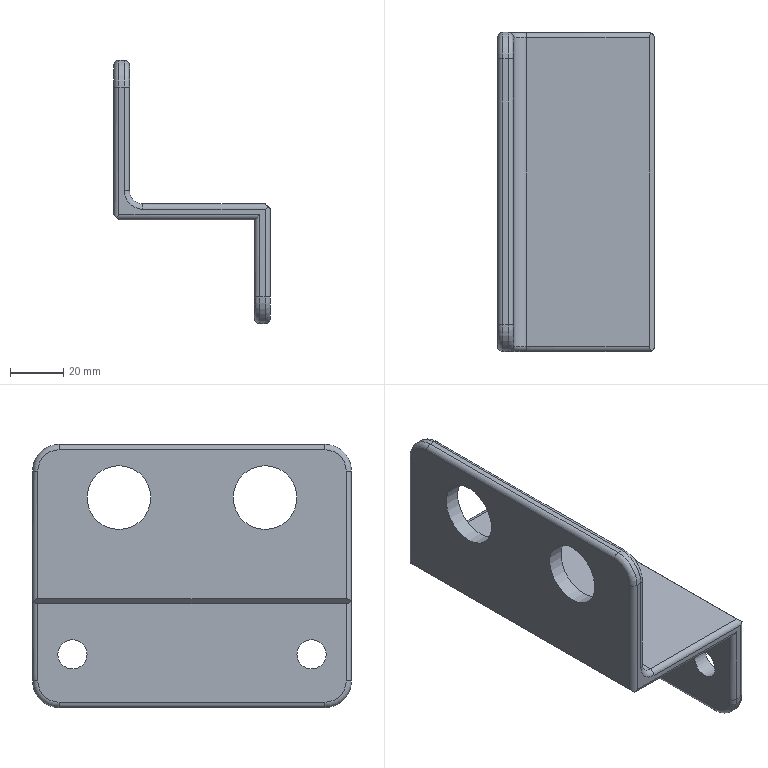Part | NX | features solid 2 | 1 solid | 47 faces | box 59 x 120 x 99 mm | volume 101632 mm3 | cylinder 25 | plane 12 | torus 10 | commonest cylinder face diameters 4 x16 20 x4 11 x2 24 x2 10 x1
STEP:
#1=CARTESIAN_POINT('',(1434.,518.,-365.));
#2=VERTEX_POINT('',#1);
#3=CARTESIAN_POINT('',(1434.,402.,-365.));
#4=VERTEX_POINT('',#3);
#5=CARTESIAN_POINT('',(1434.,460.,-365.));
#6=DIRECTION('',(0.,-1.,0.));
#7=VECTOR('',#6,1000.);
#8=LINE('',#5,#7);
#9=EDGE_CURVE('',#2,#4,#8,.T.);
#10=ORIENTED_EDGE('',*,*,#9,.F.);
#11=CARTESIAN_POINT('',(1388.,518.,-365.));
#12=VERTEX_POINT('',#11);
#13=CARTESIAN_POINT('',(1407.,518.,-365.));
#14=DIRECTION('',(1.,0.,0.));
#15=VECTOR('',#14,1000.);
#16=LINE('',#13,#15);
#17=EDGE_CURVE('',#2,#12,#16,.F.);
#18=ORIENTED_EDGE('',*,*,#17,.T.);
#19=CARTESIAN_POINT('',(1388.,402.,-365.));
#20=VERTEX_POINT('',#19);
#21=CARTESIAN_POINT('',(1388.,460.,-365.));
#22=DIRECTION('',(0.,-1.,0.));
#23=VECTOR('',#22,1000.);
#24=LINE('',#21,#23);
#25=EDGE_CURVE('',#12,#20,#24,.T.);
#26=ORIENTED_EDGE('',*,*,#25,.T.);
#27=CARTESIAN_POINT('',(1407.,402.,-365.));
#28=DIRECTION('',(-1.,0.,0.));
#29=VECTOR('',#28,1000.);
#30=LINE('',#27,#29);
#31=EDGE_CURVE('',#20,#4,#30,.F.);
#32=ORIENTED_EDGE('',*,*,#31,.T.);
#33=EDGE_LOOP('',(#10,#18,#26,#32));
#34=FACE_BOUND('',#33,.T.);
#35=CARTESIAN_POINT('',(1407.,460.,-365.));
#36=DIRECTION('',(0.,0.,1.));
#37=DIRECTION('',(0.,1.,0.));
#38=AXIS2_PLACEMENT_3D('',#35,#36,#37);
#39=PLANE('',#38);
#40=ADVANCED_FACE('',(#34),#39,.T.);
#41=CARTESIAN_POINT('',(1379.,400.,-321.));
#42=VERTEX_POINT('',#41);
#43=CARTESIAN_POINT('',(1379.,400.,-369.));
#44=VERTEX_POINT('',#43);
#45=CARTESIAN_POINT('',(1379.,400.,-371.));
#46=DIRECTION('',(0.,0.,1.));
#47=VECTOR('',#46,1000.);
#48=LINE('',#45,#47);
#49=EDGE_CURVE('',#42,#44,#48,.F.);
#50=ORIENTED_EDGE('',*,*,#49,.T.);
#51=CARTESIAN_POINT('',(1432.,400.,-369.));
#52=VERTEX_POINT('',#51);
#53=CARTESIAN_POINT('',(1407.,400.,-369.));
#54=DIRECTION('',(1.,0.,0.));
#55=VECTOR('',#54,1000.);
#56=LINE('',#53,#55);
#57=EDGE_CURVE('',#44,#52,#56,.T.);
#58=ORIENTED_EDGE('',*,*,#57,.T.);
#59=CARTESIAN_POINT('',(1432.,400.,-400.));
#60=VERTEX_POINT('',#59);
#61=CARTESIAN_POINT('',(1432.,400.,-380.));
#62=DIRECTION('',(0.,0.,1.));
#63=VECTOR('',#62,1000.);
#64=LINE('',#61,#63);
#65=EDGE_CURVE('',#60,#52,#64,.T.);
#66=ORIENTED_EDGE('',*,*,#65,.F.);
#67=CARTESIAN_POINT('',(1434.,400.,-400.));
#68=VERTEX_POINT('',#67);
#69=CARTESIAN_POINT('',(1436.,400.,-400.));
#70=DIRECTION('',(-1.,0.,0.));
#71=VECTOR('',#70,1000.);
#72=LINE('',#69,#71);
#73=EDGE_CURVE('',#68,#60,#72,.T.);
#74=ORIENTED_EDGE('',*,*,#73,.F.);
#75=CARTESIAN_POINT('',(1434.,400.,-367.));
#76=VERTEX_POINT('',#75);
#77=CARTESIAN_POINT('',(1434.,400.,-380.));
#78=DIRECTION('',(0.,0.,-1.));
#79=VECTOR('',#78,1000.);
#80=LINE('',#77,#79);
#81=EDGE_CURVE('',#76,#68,#80,.T.);
#82=ORIENTED_EDGE('',*,*,#81,.F.);
#83=CARTESIAN_POINT('',(1388.,400.,-367.));
#84=VERTEX_POINT('',#83);
#85=CARTESIAN_POINT('',(1407.,400.,-367.));
#86=DIRECTION('',(-1.,0.,0.));
#87=VECTOR('',#86,1000.);
#88=LINE('',#85,#87);
#89=EDGE_CURVE('',#76,#84,#88,.T.);
#90=ORIENTED_EDGE('',*,*,#89,.T.);
#91=CARTESIAN_POINT('',(1381.,400.,-360.));
#92=VERTEX_POINT('',#91);
#93=CARTESIAN_POINT('',(1388.,400.,-360.));
#94=DIRECTION('',(0.,-1.,0.));
#95=DIRECTION('',(0.,0.,1.));
#96=AXIS2_PLACEMENT_3D('',#93,#94,#95);
#97=CIRCLE('',#96,7.);
#98=EDGE_CURVE('',#84,#92,#97,.F.);
#99=ORIENTED_EDGE('',*,*,#98,.T.);
#100=CARTESIAN_POINT('',(1381.,400.,-321.));
#101=VERTEX_POINT('',#100);
#102=CARTESIAN_POINT('',(1381.,400.,-321.));
#103=DIRECTION('',(0.,0.,1.));
#104=VECTOR('',#103,1000.);
#105=LINE('',#102,#104);
#106=EDGE_CURVE('',#92,#101,#105,.T.);
#107=ORIENTED_EDGE('',*,*,#106,.T.);
#108=CARTESIAN_POINT('',(1407.,400.,-321.));
#109=DIRECTION('',(1.,0.,0.));
#110=VECTOR('',#109,1000.);
#111=LINE('',#108,#110);
#112=EDGE_CURVE('',#101,#42,#111,.F.);
#113=ORIENTED_EDGE('',*,*,#112,.T.);
#114=EDGE_LOOP('',(#50,#58,#66,#74,#82,#90,#99,#107,#113));
#115=FACE_BOUND('',#114,.T.);
#116=CARTESIAN_POINT('',(1407.,400.,-371.));
#117=DIRECTION('',(0.,-1.,0.));
#118=DIRECTION('',(0.,0.,1.));
#119=AXIS2_PLACEMENT_3D('',#116,#117,#118);
#120=PLANE('',#119);
#121=ADVANCED_FACE('',(#115),#120,.T.);
#122=CARTESIAN_POINT('',(1377.,432.5,-319.));
#123=VERTEX_POINT('',#122);
#124=CARTESIAN_POINT('',(1377.,432.5,-331.));
#125=DIRECTION('',(1.,0.,0.));
#126=DIRECTION('',(0.,0.,1.));
#127=AXIS2_PLACEMENT_3D('',#124,#125,#126);
#128=CIRCLE('',#127,12.);
#129=EDGE_CURVE('',#123,#123,#128,.T.);
#130=ORIENTED_EDGE('',*,*,#129,.T.);
#131=EDGE_LOOP('',(#130));
#132=FACE_BOUND('',#131,.T.);
#133=CARTESIAN_POINT('',(1377.,487.5,-319.));
#134=VERTEX_POINT('',#133);
#135=CARTESIAN_POINT('',(1377.,487.5,-331.));
#136=DIRECTION('',(-1.,0.,0.));
#137=DIRECTION('',(0.,0.,1.));
#138=AXIS2_PLACEMENT_3D('',#135,#136,#137);
#139=CIRCLE('',#138,12.);
#140=EDGE_CURVE('',#134,#134,#139,.T.);
#141=ORIENTED_EDGE('',*,*,#140,.F.);
#142=EDGE_LOOP('',(#141));
#143=FACE_BOUND('',#142,.T.);
#144=CARTESIAN_POINT('',(1377.,518.,-321.));
#145=VERTEX_POINT('',#144);
#146=CARTESIAN_POINT('',(1377.,518.,-369.));
#147=VERTEX_POINT('',#146);
#148=CARTESIAN_POINT('',(1377.,518.,-371.));
#149=DIRECTION('',(0.,0.,1.));
#150=VECTOR('',#149,1000.);
#151=LINE('',#148,#150);
#152=EDGE_CURVE('',#145,#147,#151,.F.);
#153=ORIENTED_EDGE('',*,*,#152,.T.);
#154=CARTESIAN_POINT('',(1377.,402.,-369.));
#155=VERTEX_POINT('',#154);
#156=CARTESIAN_POINT('',(1377.,460.,-369.));
#157=DIRECTION('',(0.,-1.,0.));
#158=VECTOR('',#157,1000.);
#159=LINE('',#156,#158);
#160=EDGE_CURVE('',#147,#155,#159,.T.);
#161=ORIENTED_EDGE('',*,*,#160,.T.);
#162=CARTESIAN_POINT('',(1377.,402.,-321.));
#163=VERTEX_POINT('',#162);
#164=CARTESIAN_POINT('',(1377.,402.,-371.));
#165=DIRECTION('',(0.,0.,1.));
#166=VECTOR('',#165,1000.);
#167=LINE('',#164,#166);
#168=EDGE_CURVE('',#155,#163,#167,.T.);
#169=ORIENTED_EDGE('',*,*,#168,.T.);
#170=CARTESIAN_POINT('',(1377.,410.,-313.));
#171=VERTEX_POINT('',#170);
#172=CARTESIAN_POINT('',(1377.,410.,-321.));
#173=DIRECTION('',(-1.,0.,0.));
#174=DIRECTION('',(0.,0.,1.));
#175=AXIS2_PLACEMENT_3D('',#172,#173,#174);
#176=CIRCLE('',#175,8.);
#177=EDGE_CURVE('',#163,#171,#176,.T.);
#178=ORIENTED_EDGE('',*,*,#177,.T.);
#179=CARTESIAN_POINT('',(1377.,510.,-313.));
#180=VERTEX_POINT('',#179);
#181=CARTESIAN_POINT('',(1377.,460.,-313.));
#182=DIRECTION('',(0.,1.,0.));
#183=VECTOR('',#182,1000.);
#184=LINE('',#181,#183);
#185=EDGE_CURVE('',#171,#180,#184,.T.);
#186=ORIENTED_EDGE('',*,*,#185,.T.);
#187=CARTESIAN_POINT('',(1377.,510.,-321.));
#188=DIRECTION('',(-1.,0.,0.));
#189=DIRECTION('',(0.,0.,1.));
#190=AXIS2_PLACEMENT_3D('',#187,#188,#189);
#191=CIRCLE('',#190,8.);
#192=EDGE_CURVE('',#180,#145,#191,.T.);
#193=ORIENTED_EDGE('',*,*,#192,.T.);
#194=EDGE_LOOP('',(#153,#161,#169,#178,#186,#193));
#195=FACE_BOUND('',#194,.T.);
#196=CARTESIAN_POINT('',(1377.,460.,-371.));
#197=DIRECTION('',(-1.,0.,0.));
#198=DIRECTION('',(0.,0.,1.));
#199=AXIS2_PLACEMENT_3D('',#196,#197,#198);
#200=PLANE('',#199);
#201=ADVANCED_FACE('',(#132,#143,#195),#200,.T.);
#202=CARTESIAN_POINT('',(1430.,402.,-371.));
#203=VERTEX_POINT('',#202);
#204=CARTESIAN_POINT('',(1430.,518.,-371.));
#205=VERTEX_POINT('',#204);
#206=CARTESIAN_POINT('',(1430.,460.,-371.));
#207=DIRECTION('',(0.,1.,0.));
#208=VECTOR('',#207,1000.);
#209=LINE('',#206,#208);
#210=EDGE_CURVE('',#203,#205,#209,.T.);
#211=ORIENTED_EDGE('',*,*,#210,.F.);
#212=CARTESIAN_POINT('',(1379.,402.,-371.));
#213=VERTEX_POINT('',#212);
#214=CARTESIAN_POINT('',(1407.,402.,-371.));
#215=DIRECTION('',(1.,0.,0.));
#216=VECTOR('',#215,1000.);
#217=LINE('',#214,#216);
#218=EDGE_CURVE('',#203,#213,#217,.F.);
#219=ORIENTED_EDGE('',*,*,#218,.T.);
#220=CARTESIAN_POINT('',(1379.,518.,-371.));
#221=VERTEX_POINT('',#220);
#222=CARTESIAN_POINT('',(1379.,460.,-371.));
#223=DIRECTION('',(0.,1.,0.));
#224=VECTOR('',#223,1000.);
#225=LINE('',#222,#224);
#226=EDGE_CURVE('',#213,#221,#225,.T.);
#227=ORIENTED_EDGE('',*,*,#226,.T.);
#228=CARTESIAN_POINT('',(1407.,518.,-371.));
#229=DIRECTION('',(-1.,0.,0.));
#230=VECTOR('',#229,1000.);
#231=LINE('',#228,#230);
#232=EDGE_CURVE('',#221,#205,#231,.F.);
#233=ORIENTED_EDGE('',*,*,#232,.T.);
#234=EDGE_LOOP('',(#211,#219,#227,#233));
#235=FACE_BOUND('',#234,.T.);
#236=CARTESIAN_POINT('',(1407.,460.,-371.));
#237=DIRECTION('',(0.,0.,-1.));
#238=DIRECTION('',(0.,-1.,0.));
#239=AXIS2_PLACEMENT_3D('',#236,#237,#238);
#240=PLANE('',#239);
#241=ADVANCED_FACE('',(#235),#240,.T.);
#242=CARTESIAN_POINT('',(1388.,520.,-367.));
#243=VERTEX_POINT('',#242);
#244=CARTESIAN_POINT('',(1434.,520.,-367.));
#245=VERTEX_POINT('',#244);
#246=CARTESIAN_POINT('',(1407.,520.,-367.));
#247=DIRECTION('',(1.,0.,0.));
#248=VECTOR('',#247,1000.);
#249=LINE('',#246,#248);
#250=EDGE_CURVE('',#243,#245,#249,.T.);
#251=ORIENTED_EDGE('',*,*,#250,.T.);
#252=CARTESIAN_POINT('',(1434.,520.,-400.));
#253=VERTEX_POINT('',#252);
#254=CARTESIAN_POINT('',(1434.,520.,-380.));
#255=DIRECTION('',(0.,0.,1.));
#256=VECTOR('',#255,1000.);
#257=LINE('',#254,#256);
#258=EDGE_CURVE('',#253,#245,#257,.T.);
#259=ORIENTED_EDGE('',*,*,#258,.F.);
#260=CARTESIAN_POINT('',(1432.,520.,-400.));
#261=VERTEX_POINT('',#260);
#262=CARTESIAN_POINT('',(1436.,520.,-400.));
#263=DIRECTION('',(-1.,0.,0.));
#264=VECTOR('',#263,1000.);
#265=LINE('',#262,#264);
#266=EDGE_CURVE('',#261,#253,#265,.F.);
#267=ORIENTED_EDGE('',*,*,#266,.F.);
#268=CARTESIAN_POINT('',(1432.,520.,-369.));
#269=VERTEX_POINT('',#268);
#270=CARTESIAN_POINT('',(1432.,520.,-380.));
#271=DIRECTION('',(0.,0.,-1.));
#272=VECTOR('',#271,1000.);
#273=LINE('',#270,#272);
#274=EDGE_CURVE('',#269,#261,#273,.T.);
#275=ORIENTED_EDGE('',*,*,#274,.F.);
#276=CARTESIAN_POINT('',(1379.,520.,-369.));
#277=VERTEX_POINT('',#276);
#278=CARTESIAN_POINT('',(1407.,520.,-369.));
#279=DIRECTION('',(-1.,0.,0.));
#280=VECTOR('',#279,1000.);
#281=LINE('',#278,#280);
#282=EDGE_CURVE('',#269,#277,#281,.T.);
#283=ORIENTED_EDGE('',*,*,#282,.T.);
#284=CARTESIAN_POINT('',(1379.,520.,-321.));
#285=VERTEX_POINT('',#284);
#286=CARTESIAN_POINT('',(1379.,520.,-371.));
#287=DIRECTION('',(0.,0.,1.));
#288=VECTOR('',#287,1000.);
#289=LINE('',#286,#288);
#290=EDGE_CURVE('',#277,#285,#289,.T.);
#291=ORIENTED_EDGE('',*,*,#290,.T.);
#292=CARTESIAN_POINT('',(1381.,520.,-321.));
#293=VERTEX_POINT('',#292);
#294=CARTESIAN_POINT('',(1407.,520.,-321.));
#295=DIRECTION('',(1.,0.,0.));
#296=VECTOR('',#295,1000.);
#297=LINE('',#294,#296);
#298=EDGE_CURVE('',#285,#293,#297,.T.);
#299=ORIENTED_EDGE('',*,*,#298,.T.);
#300=CARTESIAN_POINT('',(1381.,520.,-360.));
#301=VERTEX_POINT('',#300);
#302=CARTESIAN_POINT('',(1381.,520.,-360.));
#303=DIRECTION('',(0.,0.,1.));
#304=VECTOR('',#303,1000.);
#305=LINE('',#302,#304);
#306=EDGE_CURVE('',#293,#301,#305,.F.);
#307=ORIENTED_EDGE('',*,*,#306,.T.);
#308=CARTESIAN_POINT('',(1388.,520.,-360.));
#309=DIRECTION('',(0.,1.,0.));
#310=DIRECTION('',(0.,0.,-1.));
#311=AXIS2_PLACEMENT_3D('',#308,#309,#310);
#312=CIRCLE('',#311,7.);
#313=EDGE_CURVE('',#301,#243,#312,.F.);
#314=ORIENTED_EDGE('',*,*,#313,.T.);
#315=EDGE_LOOP('',(#251,#259,#267,#275,#283,#291,#299,#307,#314));
#316=FACE_BOUND('',#315,.T.);
#317=CARTESIAN_POINT('',(1407.,520.,-371.));
#318=DIRECTION('',(0.,1.,0.));
#319=DIRECTION('',(0.,0.,-1.));
#320=AXIS2_PLACEMENT_3D('',#317,#318,#319);
#321=PLANE('',#320);
#322=ADVANCED_FACE('',(#316),#321,.T.);
#323=CARTESIAN_POINT('',(1381.,510.,-311.));
#324=VERTEX_POINT('',#323);
#325=CARTESIAN_POINT('',(1379.,510.,-311.));
#326=VERTEX_POINT('',#325);
#327=CARTESIAN_POINT('',(1377.,510.,-311.));
#328=DIRECTION('',(-1.,0.,0.));
#329=VECTOR('',#328,1000.);
#330=LINE('',#327,#329);
#331=EDGE_CURVE('',#324,#326,#330,.T.);
#332=ORIENTED_EDGE('',*,*,#331,.T.);
#333=CARTESIAN_POINT('',(1379.,410.,-311.));
#334=VERTEX_POINT('',#333);
#335=CARTESIAN_POINT('',(1379.,520.,-311.));
#336=DIRECTION('',(0.,-1.,0.));
#337=VECTOR('',#336,1000.);
#338=LINE('',#335,#337);
#339=EDGE_CURVE('',#326,#334,#338,.T.);
#340=ORIENTED_EDGE('',*,*,#339,.T.);
#341=CARTESIAN_POINT('',(1381.,410.,-311.));
#342=VERTEX_POINT('',#341);
#343=CARTESIAN_POINT('',(1377.,410.,-311.));
#344=DIRECTION('',(-1.,0.,0.));
#345=VECTOR('',#344,1000.);
#346=LINE('',#343,#345);
#347=EDGE_CURVE('',#334,#342,#346,.F.);
#348=ORIENTED_EDGE('',*,*,#347,.T.);
#349=CARTESIAN_POINT('',(1381.,510.,-311.));
#350=DIRECTION('',(0.,-1.,0.));
#351=VECTOR('',#350,1000.);
#352=LINE('',#349,#351);
#353=EDGE_CURVE('',#342,#324,#352,.F.);
#354=ORIENTED_EDGE('',*,*,#353,.T.);
#355=EDGE_LOOP('',(#332,#340,#348,#354));
#356=FACE_BOUND('',#355,.T.);
#357=CARTESIAN_POINT('',(1377.,520.,-311.));
#358=DIRECTION('',(0.,0.,-1.));
#359=DIRECTION('',(0.,-1.,0.));
#360=AXIS2_PLACEMENT_3D('',#357,#358,#359);
#361=PLANE('',#360);
#362=ADVANCED_FACE('',(#356),#361,.F.);
#363=CARTESIAN_POINT('',(1383.,432.5,-319.));
#364=VERTEX_POINT('',#363);
#365=CARTESIAN_POINT('',(1383.,432.5,-331.));
#366=DIRECTION('',(1.,0.,0.));
#367=DIRECTION('',(0.,0.,1.));
#368=AXIS2_PLACEMENT_3D('',#365,#366,#367);
#369=CIRCLE('',#368,12.);
#370=EDGE_CURVE('',#364,#364,#369,.T.);
#371=ORIENTED_EDGE('',*,*,#370,.F.);
#372=EDGE_LOOP('',(#371));
#373=FACE_BOUND('',#372,.T.);
#374=CARTESIAN_POINT('',(1383.,487.5,-319.));
#375=VERTEX_POINT('',#374);
#376=CARTESIAN_POINT('',(1383.,487.5,-331.));
#377=DIRECTION('',(-1.,0.,0.));
#378=DIRECTION('',(0.,0.,1.));
#379=AXIS2_PLACEMENT_3D('',#376,#377,#378);
#380=CIRCLE('',#379,12.);
#381=EDGE_CURVE('',#375,#375,#380,.T.);
#382=ORIENTED_EDGE('',*,*,#381,.T.);
#383=EDGE_LOOP('',(#382));
#384=FACE_BOUND('',#383,.T.);
#385=CARTESIAN_POINT('',(1383.,410.,-313.));
#386=VERTEX_POINT('',#385);
#387=CARTESIAN_POINT('',(1383.,402.,-321.));
#388=VERTEX_POINT('',#387);
#389=CARTESIAN_POINT('',(1383.,410.,-321.));
#390=DIRECTION('',(-1.,0.,0.));
#391=DIRECTION('',(0.,0.,1.));
#392=AXIS2_PLACEMENT_3D('',#389,#390,#391);
#393=CIRCLE('',#392,8.);
#394=EDGE_CURVE('',#386,#388,#393,.F.);
#395=ORIENTED_EDGE('',*,*,#394,.T.);
#396=CARTESIAN_POINT('',(1383.,402.,-360.));
#397=VERTEX_POINT('',#396);
#398=CARTESIAN_POINT('',(1383.,402.,-360.));
#399=DIRECTION('',(0.,0.,1.));
#400=VECTOR('',#399,1000.);
#401=LINE('',#398,#400);
#402=EDGE_CURVE('',#388,#397,#401,.F.);
#403=ORIENTED_EDGE('',*,*,#402,.T.);
#404=CARTESIAN_POINT('',(1383.,518.,-360.));
#405=VERTEX_POINT('',#404);
#406=CARTESIAN_POINT('',(1383.,520.,-360.));
#407=DIRECTION('',(0.,-1.,0.));
#408=VECTOR('',#407,1000.);
#409=LINE('',#406,#408);
#410=EDGE_CURVE('',#397,#405,#409,.F.);
#411=ORIENTED_EDGE('',*,*,#410,.T.);
#412=CARTESIAN_POINT('',(1383.,518.,-321.));
#413=VERTEX_POINT('',#412);
#414=CARTESIAN_POINT('',(1383.,518.,-321.));
#415=DIRECTION('',(0.,0.,1.));
#416=VECTOR('',#415,1000.);
#417=LINE('',#414,#416);
#418=EDGE_CURVE('',#405,#413,#417,.T.);
#419=ORIENTED_EDGE('',*,*,#418,.T.);
#420=CARTESIAN_POINT('',(1383.,510.,-313.));
#421=VERTEX_POINT('',#420);
#422=CARTESIAN_POINT('',(1383.,510.,-321.));
#423=DIRECTION('',(-1.,0.,0.));
#424=DIRECTION('',(0.,0.,1.));
#425=AXIS2_PLACEMENT_3D('',#422,#423,#424);
#426=CIRCLE('',#425,8.);
#427=EDGE_CURVE('',#413,#421,#426,.F.);
#428=ORIENTED_EDGE('',*,*,#427,.T.);
#429=CARTESIAN_POINT('',(1383.,410.,-313.));
#430=DIRECTION('',(0.,1.,0.));
#431=VECTOR('',#430,1000.);
#432=LINE('',#429,#431);
#433=EDGE_CURVE('',#421,#386,#432,.F.);
#434=ORIENTED_EDGE('',*,*,#433,.T.);
#435=EDGE_LOOP('',(#395,#403,#411,#419,#428,#434));
#436=FACE_BOUND('',#435,.T.);
#437=CARTESIAN_POINT('',(1383.,520.,-371.));
#438=DIRECTION('',(-1.,0.,0.));
#439=DIRECTION('',(0.,0.,1.));
#440=AXIS2_PLACEMENT_3D('',#437,#438,#439);
#441=PLANE('',#440);
#442=ADVANCED_FACE('',(#373,#384,#436),#441,.F.);
#443=ORIENTED_EDGE('',*,*,#298,.F.);
#444=CARTESIAN_POINT('',(1379.,510.,-321.));
#445=DIRECTION('',(-1.,0.,0.));
#446=DIRECTION('',(0.,0.,1.));
#447=AXIS2_PLACEMENT_3D('',#444,#445,#446);
#448=CIRCLE('',#447,10.);
#449=EDGE_CURVE('',#285,#326,#448,.F.);
#450=ORIENTED_EDGE('',*,*,#449,.T.);
#451=ORIENTED_EDGE('',*,*,#331,.F.);
#452=CARTESIAN_POINT('',(1381.,510.,-321.));
#453=DIRECTION('',(-1.,0.,0.));
#454=DIRECTION('',(0.,0.,1.));
#455=AXIS2_PLACEMENT_3D('',#452,#453,#454);
#456=CIRCLE('',#455,10.);
#457=EDGE_CURVE('',#324,#293,#456,.T.);
#458=ORIENTED_EDGE('',*,*,#457,.T.);
#459=EDGE_LOOP('',(#443,#450,#451,#458));
#460=FACE_BOUND('',#459,.T.);
#461=CARTESIAN_POINT('',(1377.,510.,-321.));
#462=DIRECTION('',(1.,0.,0.));
#463=DIRECTION('',(0.,0.,-1.));
#464=AXIS2_PLACEMENT_3D('',#461,#462,#463);
#465=CYLINDRICAL_SURFACE('',#464,10.);
#466=ADVANCED_FACE('',(#460),#465,.T.);
#467=ORIENTED_EDGE('',*,*,#347,.F.);
#468=CARTESIAN_POINT('',(1379.,410.,-321.));
#469=DIRECTION('',(-1.,0.,0.));
#470=DIRECTION('',(0.,0.,1.));
#471=AXIS2_PLACEMENT_3D('',#468,#469,#470);
#472=CIRCLE('',#471,10.);
#473=EDGE_CURVE('',#334,#42,#472,.F.);
#474=ORIENTED_EDGE('',*,*,#473,.T.);
#475=ORIENTED_EDGE('',*,*,#112,.F.);
#476=CARTESIAN_POINT('',(1381.,410.,-321.));
#477=DIRECTION('',(-1.,0.,0.));
#478=DIRECTION('',(0.,0.,1.));
#479=AXIS2_PLACEMENT_3D('',#476,#477,#478);
#480=CIRCLE('',#479,10.);
#481=EDGE_CURVE('',#101,#342,#480,.T.);
#482=ORIENTED_EDGE('',*,*,#481,.T.);
#483=EDGE_LOOP('',(#467,#474,#475,#482));
#484=FACE_BOUND('',#483,.T.);
#485=CARTESIAN_POINT('',(1407.,410.,-321.));
#486=DIRECTION('',(1.,0.,0.));
#487=DIRECTION('',(0.,0.,-1.));
#488=AXIS2_PLACEMENT_3D('',#485,#486,#487);
#489=CYLINDRICAL_SURFACE('',#488,10.);
#490=ADVANCED_FACE('',(#484),#489,.T.);
#491=ORIENTED_EDGE('',*,*,#410,.F.);
#492=CARTESIAN_POINT('',(1388.,402.,-360.));
#493=DIRECTION('',(0.,-1.,0.));
#494=DIRECTION('',(0.,0.,1.));
#495=AXIS2_PLACEMENT_3D('',#492,#493,#494);
#496=CIRCLE('',#495,5.);
#497=EDGE_CURVE('',#397,#20,#496,.T.);
#498=ORIENTED_EDGE('',*,*,#497,.T.);
#499=ORIENTED_EDGE('',*,*,#25,.F.);
#500=CARTESIAN_POINT('',(1388.,518.,-360.));
#501=DIRECTION('',(0.,1.,0.));
#502=DIRECTION('',(0.,0.,-1.));
#503=AXIS2_PLACEMENT_3D('',#500,#501,#502);
#504=CIRCLE('',#503,5.);
#505=EDGE_CURVE('',#12,#405,#504,.T.);
#506=ORIENTED_EDGE('',*,*,#505,.T.);
#507=EDGE_LOOP('',(#491,#498,#499,#506));
#508=FACE_BOUND('',#507,.T.);
#509=CARTESIAN_POINT('',(1388.,460.,-360.));
#510=DIRECTION('',(0.,-1.,0.));
#511=DIRECTION('',(0.,0.,1.));
#512=AXIS2_PLACEMENT_3D('',#509,#510,#511);
#513=CYLINDRICAL_SURFACE('',#512,5.);
#514=ADVANCED_FACE('',(#508),#513,.F.);
#515=CARTESIAN_POINT('',(1378.,519.732,-370.));
#516=VERTEX_POINT('',#515);
#517=CARTESIAN_POINT('',(1379.,518.,-369.));
#518=DIRECTION('',(-0.7071,0.,0.7071));
#519=DIRECTION('',(0.7071,0.,0.7071));
#520=AXIS2_PLACEMENT_3D('',#517,#518,#519);
#521=ELLIPSE('',#520,2.828,2.);
#522=EDGE_CURVE('',#516,#277,#521,.F.);
#523=ORIENTED_EDGE('',*,*,#522,.F.);
#524=CARTESIAN_POINT('',(1379.,518.,-371.));
#525=DIRECTION('',(0.7071,0.,0.7071));
#526=DIRECTION('',(-0.7071,0.,0.7071));
#527=AXIS2_PLACEMENT_3D('',#524,#525,#526);
#528=ELLIPSE('',#527,2.828,2.);
#529=EDGE_CURVE('',#516,#147,#528,.T.);
#530=ORIENTED_EDGE('',*,*,#529,.T.);
#531=ORIENTED_EDGE('',*,*,#152,.F.);
#532=CARTESIAN_POINT('',(1379.,518.,-321.));
#533=DIRECTION('',(0.,0.,1.));
#534=DIRECTION('',(0.,1.,0.));
#535=AXIS2_PLACEMENT_3D('',#532,#533,#534);
#536=CIRCLE('',#535,2.);
#537=EDGE_CURVE('',#285,#145,#536,.T.);
#538=ORIENTED_EDGE('',*,*,#537,.F.);
#539=ORIENTED_EDGE('',*,*,#290,.F.);
#540=EDGE_LOOP('',(#523,#530,#531,#538,#539));
#541=FACE_BOUND('',#540,.T.);
#542=CARTESIAN_POINT('',(1379.,518.,-371.));
#543=DIRECTION('',(0.,0.,1.));
#544=DIRECTION('',(0.,1.,0.));
#545=AXIS2_PLACEMENT_3D('',#542,#543,#544);
#546=CYLINDRICAL_SURFACE('',#545,2.);
#547=ADVANCED_FACE('',(#541),#546,.T.);
#548=ORIENTED_EDGE('',*,*,#537,.T.);
#549=ORIENTED_EDGE('',*,*,#192,.F.);
#550=CARTESIAN_POINT('',(1379.,510.,-313.));
#551=DIRECTION('',(0.,-1.,0.));
#552=DIRECTION('',(0.,0.,1.));
#553=AXIS2_PLACEMENT_3D('',#550,#551,#552);
#554=CIRCLE('',#553,2.);
#555=EDGE_CURVE('',#326,#180,#554,.T.);
#556=ORIENTED_EDGE('',*,*,#555,.F.);
#557=ORIENTED_EDGE('',*,*,#449,.F.);
#558=EDGE_LOOP('',(#548,#549,#556,#557));
#559=FACE_BOUND('',#558,.T.);
#560=CARTESIAN_POINT('',(1379.,510.,-321.));
#561=DIRECTION('',(-1.,0.,0.));
#562=DIRECTION('',(0.,0.,1.));
#563=AXIS2_PLACEMENT_3D('',#560,#561,#562);
#564=TOROIDAL_SURFACE('',#563,8.,2.);
#565=ADVANCED_FACE('',(#559),#564,.T.);
#566=CARTESIAN_POINT('',(1432.,518.,-369.));
#567=DIRECTION('',(-0.7071,0.,0.7071));
#568=DIRECTION('',(-0.7071,0.,-0.7071));
#569=AXIS2_PLACEMENT_3D('',#566,#567,#568);
#570=ELLIPSE('',#569,2.828,2.);
#571=EDGE_CURVE('',#205,#269,#570,.F.);
#572=ORIENTED_EDGE('',*,*,#571,.F.);
#573=ORIENTED_EDGE('',*,*,#232,.F.);
#574=CARTESIAN_POINT('',(1377.,518.,-369.));
#575=DIRECTION('',(0.7071,0.,0.7071));
#576=DIRECTION('',(-0.7071,0.,0.7071));
#577=AXIS2_PLACEMENT_3D('',#574,#575,#576);
#578=ELLIPSE('',#577,2.828,2.);
#579=EDGE_CURVE('',#221,#516,#578,.T.);
#580=ORIENTED_EDGE('',*,*,#579,.T.);
#581=ORIENTED_EDGE('',*,*,#522,.T.);
#582=ORIENTED_EDGE('',*,*,#282,.F.);
#583=EDGE_LOOP('',(#572,#573,#580,#581,#582));
#584=FACE_BOUND('',#583,.T.);
#585=CARTESIAN_POINT('',(1407.,518.,-369.));
#586=DIRECTION('',(-1.,0.,0.));
#587=DIRECTION('',(0.,0.,1.));
#588=AXIS2_PLACEMENT_3D('',#585,#586,#587);
#589=CYLINDRICAL_SURFACE('',#588,2.);
#590=ADVANCED_FACE('',(#584),#589,.T.);
#591=ORIENTED_EDGE('',*,*,#555,.T.);
#592=ORIENTED_EDGE('',*,*,#185,.F.);
#593=CARTESIAN_POINT('',(1379.,410.,-313.));
#594=DIRECTION('',(0.,-1.,0.));
#595=DIRECTION('',(0.,0.,1.));
#596=AXIS2_PLACEMENT_3D('',#593,#594,#595);
#597=CIRCLE('',#596,2.);
#598=EDGE_CURVE('',#334,#171,#597,.T.);
#599=ORIENTED_EDGE('',*,*,#598,.F.);
#600=ORIENTED_EDGE('',*,*,#339,.F.);
#601=EDGE_LOOP('',(#591,#592,#599,#600));
#602=FACE_BOUND('',#601,.T.);
#603=CARTESIAN_POINT('',(1379.,520.,-313.));
#604=DIRECTION('',(0.,1.,0.));
#605=DIRECTION('',(0.,0.,-1.));
#606=AXIS2_PLACEMENT_3D('',#603,#604,#605);
#607=CYLINDRICAL_SURFACE('',#606,2.);
#608=ADVANCED_FACE('',(#602),#607,.T.);
#609=ORIENTED_EDGE('',*,*,#598,.T.);
#610=ORIENTED_EDGE('',*,*,#177,.F.);
#611=CARTESIAN_POINT('',(1379.,402.,-321.));
#612=DIRECTION('',(0.,0.,-1.));
#613=DIRECTION('',(0.,-1.,0.));
#614=AXIS2_PLACEMENT_3D('',#611,#612,#613);
#615=CIRCLE('',#614,2.);
#616=EDGE_CURVE('',#42,#163,#615,.T.);
#617=ORIENTED_EDGE('',*,*,#616,.F.);
#618=ORIENTED_EDGE('',*,*,#473,.F.);
#619=EDGE_LOOP('',(#609,#610,#617,#618));
#620=FACE_BOUND('',#619,.T.);
#621=CARTESIAN_POINT('',(1379.,410.,-321.));
#622=DIRECTION('',(-1.,0.,0.));
#623=DIRECTION('',(0.,0.,1.));
#624=AXIS2_PLACEMENT_3D('',#621,#622,#623);
#625=TOROIDAL_SURFACE('',#624,8.,2.);
#626=ADVANCED_FACE('',(#620),#625,.T.);
#627=ORIENTED_EDGE('',*,*,#168,.F.);
#628=CARTESIAN_POINT('',(1378.,400.268,-370.));
#629=VERTEX_POINT('',#628);
#630=CARTESIAN_POINT('',(1379.,402.,-371.));
#631=DIRECTION('',(0.7071,0.,0.7071));
#632=DIRECTION('',(-0.7071,0.,0.7071));
#633=AXIS2_PLACEMENT_3D('',#630,#631,#632);
#634=ELLIPSE('',#633,2.828,2.);
#635=EDGE_CURVE('',#155,#629,#634,.T.);
#636=ORIENTED_EDGE('',*,*,#635,.T.);
#637=CARTESIAN_POINT('',(1379.,402.,-369.));
#638=DIRECTION('',(-0.7071,0.,0.7071));
#639=DIRECTION('',(0.7071,0.,0.7071));
#640=AXIS2_PLACEMENT_3D('',#637,#638,#639);
#641=ELLIPSE('',#640,2.828,2.);
#642=EDGE_CURVE('',#44,#629,#641,.F.);
#643=ORIENTED_EDGE('',*,*,#642,.F.);
#644=ORIENTED_EDGE('',*,*,#49,.F.);
#645=ORIENTED_EDGE('',*,*,#616,.T.);
#646=EDGE_LOOP('',(#627,#636,#643,#644,#645));
#647=FACE_BOUND('',#646,.T.);
#648=CARTESIAN_POINT('',(1379.,402.,-371.));
#649=DIRECTION('',(0.,0.,1.));
#650=DIRECTION('',(0.,1.,0.));
#651=AXIS2_PLACEMENT_3D('',#648,#649,#650);
#652=CYLINDRICAL_SURFACE('',#651,2.);
#653=ADVANCED_FACE('',(#647),#652,.T.);
#654=CARTESIAN_POINT('',(1432.,402.,-369.));
#655=DIRECTION('',(0.7071,0.,-0.7071));
#656=DIRECTION('',(0.7071,0.,0.7071));
#657=AXIS2_PLACEMENT_3D('',#654,#655,#656);
#658=ELLIPSE('',#657,2.828,2.);
#659=EDGE_CURVE('',#52,#203,#658,.T.);
#660=ORIENTED_EDGE('',*,*,#659,.F.);
#661=ORIENTED_EDGE('',*,*,#57,.F.);
#662=ORIENTED_EDGE('',*,*,#642,.T.);
#663=CARTESIAN_POINT('',(1377.,402.,-369.));
#664=DIRECTION('',(0.7071,0.,0.7071));
#665=DIRECTION('',(0.7071,0.,-0.7071));
#666=AXIS2_PLACEMENT_3D('',#663,#664,#665);
#667=ELLIPSE('',#666,2.828,2.);
#668=EDGE_CURVE('',#629,#213,#667,.T.);
#669=ORIENTED_EDGE('',*,*,#668,.T.);
#670=ORIENTED_EDGE('',*,*,#218,.F.);
#671=EDGE_LOOP('',(#660,#661,#662,#669,#670));
#672=FACE_BOUND('',#671,.T.);
#673=CARTESIAN_POINT('',(1407.,402.,-369.));
#674=DIRECTION('',(1.,0.,0.));
#675=DIRECTION('',(0.,0.,-1.));
#676=AXIS2_PLACEMENT_3D('',#673,#674,#675);
#677=CYLINDRICAL_SURFACE('',#676,2.);
#678=ADVANCED_FACE('',(#672),#677,.T.);
#679=ORIENTED_EDGE('',*,*,#17,.F.);
#680=CARTESIAN_POINT('',(1435.,519.732,-366.));
#681=VERTEX_POINT('',#680);
#682=CARTESIAN_POINT('',(1436.,518.,-367.));
#683=DIRECTION('',(-0.7071,0.,-0.7071));
#684=DIRECTION('',(0.7071,0.,-0.7071));
#685=AXIS2_PLACEMENT_3D('',#682,#683,#684);
#686=ELLIPSE('',#685,2.828,2.);
#687=EDGE_CURVE('',#2,#681,#686,.T.);
#688=ORIENTED_EDGE('',*,*,#687,.T.);
#689=CARTESIAN_POINT('',(1434.,518.,-367.));
#690=DIRECTION('',(-0.7071,0.,0.7071));
#691=DIRECTION('',(0.7071,0.,0.7071));
#692=AXIS2_PLACEMENT_3D('',#689,#690,#691);
#693=ELLIPSE('',#692,2.828,2.);
#694=EDGE_CURVE('',#245,#681,#693,.F.);
#695=ORIENTED_EDGE('',*,*,#694,.F.);
#696=ORIENTED_EDGE('',*,*,#250,.F.);
#697=CARTESIAN_POINT('',(1388.,518.,-367.));
#698=DIRECTION('',(-1.,0.,0.));
#699=DIRECTION('',(0.,0.,1.));
#700=AXIS2_PLACEMENT_3D('',#697,#698,#699);
#701=CIRCLE('',#700,2.);
#702=EDGE_CURVE('',#12,#243,#701,.T.);
#703=ORIENTED_EDGE('',*,*,#702,.F.);
#704=EDGE_LOOP('',(#679,#688,#695,#696,#703));
#705=FACE_BOUND('',#704,.T.);
#706=CARTESIAN_POINT('',(1407.,518.,-367.));
#707=DIRECTION('',(1.,0.,0.));
#708=DIRECTION('',(0.,0.,-1.));
#709=AXIS2_PLACEMENT_3D('',#706,#707,#708);
#710=CYLINDRICAL_SURFACE('',#709,2.);
#711=ADVANCED_FACE('',(#705),#710,.T.);
#712=ORIENTED_EDGE('',*,*,#702,.T.);
#713=ORIENTED_EDGE('',*,*,#313,.F.);
#714=CARTESIAN_POINT('',(1381.,518.,-360.));
#715=DIRECTION('',(0.,0.,1.));
#716=DIRECTION('',(0.,1.,0.));
#717=AXIS2_PLACEMENT_3D('',#714,#715,#716);
#718=CIRCLE('',#717,2.);
#719=EDGE_CURVE('',#405,#301,#718,.T.);
#720=ORIENTED_EDGE('',*,*,#719,.F.);
#721=ORIENTED_EDGE('',*,*,#505,.F.);
#722=EDGE_LOOP('',(#712,#713,#720,#721));
#723=FACE_BOUND('',#722,.T.);
#724=CARTESIAN_POINT('',(1388.,518.,-360.));
#725=DIRECTION('',(0.,1.,0.));
#726=DIRECTION('',(0.,0.,-1.));
#727=AXIS2_PLACEMENT_3D('',#724,#725,#726);
#728=TOROIDAL_SURFACE('',#727,7.,2.);
#729=ADVANCED_FACE('',(#723),#728,.T.);
#730=ORIENTED_EDGE('',*,*,#719,.T.);
#731=ORIENTED_EDGE('',*,*,#306,.F.);
#732=CARTESIAN_POINT('',(1381.,518.,-321.));
#733=DIRECTION('',(0.,0.,1.));
#734=DIRECTION('',(0.,1.,0.));
#735=AXIS2_PLACEMENT_3D('',#732,#733,#734);
#736=CIRCLE('',#735,2.);
#737=EDGE_CURVE('',#413,#293,#736,.T.);
#738=ORIENTED_EDGE('',*,*,#737,.F.);
#739=ORIENTED_EDGE('',*,*,#418,.F.);
#740=EDGE_LOOP('',(#730,#731,#738,#739));
#741=FACE_BOUND('',#740,.T.);
#742=CARTESIAN_POINT('',(1381.,518.,-371.));
#743=DIRECTION('',(0.,0.,-1.));
#744=DIRECTION('',(0.,-1.,0.));
#745=AXIS2_PLACEMENT_3D('',#742,#743,#744);
#746=CYLINDRICAL_SURFACE('',#745,2.);
#747=ADVANCED_FACE('',(#741),#746,.T.);
#748=ORIENTED_EDGE('',*,*,#89,.F.);
#749=CARTESIAN_POINT('',(1435.,400.268,-366.));
#750=VERTEX_POINT('',#749);
#751=CARTESIAN_POINT('',(1434.,402.,-367.));
#752=DIRECTION('',(-0.7071,0.,0.7071));
#753=DIRECTION('',(-0.7071,0.,-0.7071));
#754=AXIS2_PLACEMENT_3D('',#751,#752,#753);
#755=ELLIPSE('',#754,2.828,2.);
#756=EDGE_CURVE('',#76,#750,#755,.T.);
#757=ORIENTED_EDGE('',*,*,#756,.T.);
#758=CARTESIAN_POINT('',(1436.,402.,-367.));
#759=DIRECTION('',(-0.7071,0.,-0.7071));
#760=DIRECTION('',(-0.7071,0.,0.7071));
#761=AXIS2_PLACEMENT_3D('',#758,#759,#760);
#762=ELLIPSE('',#761,2.828,2.);
#763=EDGE_CURVE('',#750,#4,#762,.T.);
#764=ORIENTED_EDGE('',*,*,#763,.T.);
#765=ORIENTED_EDGE('',*,*,#31,.F.);
#766=CARTESIAN_POINT('',(1388.,402.,-367.));
#767=DIRECTION('',(-1.,0.,0.));
#768=DIRECTION('',(0.,0.,1.));
#769=AXIS2_PLACEMENT_3D('',#766,#767,#768);
#770=CIRCLE('',#769,2.);
#771=EDGE_CURVE('',#84,#20,#770,.T.);
#772=ORIENTED_EDGE('',*,*,#771,.F.);
#773=EDGE_LOOP('',(#748,#757,#764,#765,#772));
#774=FACE_BOUND('',#773,.T.);
#775=CARTESIAN_POINT('',(1407.,402.,-367.));
#776=DIRECTION('',(-1.,0.,0.));
#777=DIRECTION('',(0.,0.,1.));
#778=AXIS2_PLACEMENT_3D('',#775,#776,#777);
#779=CYLINDRICAL_SURFACE('',#778,2.);
#780=ADVANCED_FACE('',(#774),#779,.T.);
#781=ORIENTED_EDGE('',*,*,#737,.T.);
#782=ORIENTED_EDGE('',*,*,#457,.F.);
#783=CARTESIAN_POINT('',(1381.,510.,-313.));
#784=DIRECTION('',(0.,-1.,0.));
#785=DIRECTION('',(0.,0.,1.));
#786=AXIS2_PLACEMENT_3D('',#783,#784,#785);
#787=CIRCLE('',#786,2.);
#788=EDGE_CURVE('',#421,#324,#787,.T.);
#789=ORIENTED_EDGE('',*,*,#788,.F.);
#790=ORIENTED_EDGE('',*,*,#427,.F.);
#791=EDGE_LOOP('',(#781,#782,#789,#790));
#792=FACE_BOUND('',#791,.T.);
#793=CARTESIAN_POINT('',(1381.,510.,-321.));
#794=DIRECTION('',(-1.,0.,0.));
#795=DIRECTION('',(0.,0.,1.));
#796=AXIS2_PLACEMENT_3D('',#793,#794,#795);
#797=TOROIDAL_SURFACE('',#796,8.,2.);
#798=ADVANCED_FACE('',(#792),#797,.T.);
#799=ORIENTED_EDGE('',*,*,#771,.T.);
#800=ORIENTED_EDGE('',*,*,#497,.F.);
#801=CARTESIAN_POINT('',(1381.,402.,-360.));
#802=DIRECTION('',(0.,0.,1.));
#803=DIRECTION('',(0.,1.,0.));
#804=AXIS2_PLACEMENT_3D('',#801,#802,#803);
#805=CIRCLE('',#804,2.);
#806=EDGE_CURVE('',#92,#397,#805,.T.);
#807=ORIENTED_EDGE('',*,*,#806,.F.);
#808=ORIENTED_EDGE('',*,*,#98,.F.);
#809=EDGE_LOOP('',(#799,#800,#807,#808));
#810=FACE_BOUND('',#809,.T.);
#811=CARTESIAN_POINT('',(1388.,402.,-360.));
#812=DIRECTION('',(0.,-1.,0.));
#813=DIRECTION('',(0.,0.,1.));
#814=AXIS2_PLACEMENT_3D('',#811,#812,#813);
#815=TOROIDAL_SURFACE('',#814,7.,2.);
#816=ADVANCED_FACE('',(#810),#815,.T.);
#817=ORIENTED_EDGE('',*,*,#788,.T.);
#818=ORIENTED_EDGE('',*,*,#353,.F.);
#819=CARTESIAN_POINT('',(1381.,410.,-313.));
#820=DIRECTION('',(0.,-1.,0.));
#821=DIRECTION('',(0.,0.,1.));
#822=AXIS2_PLACEMENT_3D('',#819,#820,#821);
#823=CIRCLE('',#822,2.);
#824=EDGE_CURVE('',#386,#342,#823,.T.);
#825=ORIENTED_EDGE('',*,*,#824,.F.);
#826=ORIENTED_EDGE('',*,*,#433,.F.);
#827=EDGE_LOOP('',(#817,#818,#825,#826));
#828=FACE_BOUND('',#827,.T.);
#829=CARTESIAN_POINT('',(1381.,520.,-313.));
#830=DIRECTION('',(0.,-1.,0.));
#831=DIRECTION('',(0.,0.,1.));
#832=AXIS2_PLACEMENT_3D('',#829,#830,#831);
#833=CYLINDRICAL_SURFACE('',#832,2.);
#834=ADVANCED_FACE('',(#828),#833,.T.);
#835=ORIENTED_EDGE('',*,*,#806,.T.);
#836=ORIENTED_EDGE('',*,*,#402,.F.);
#837=CARTESIAN_POINT('',(1381.,402.,-321.));
#838=DIRECTION('',(0.,0.,1.));
#839=DIRECTION('',(0.,1.,0.));
#840=AXIS2_PLACEMENT_3D('',#837,#838,#839);
#841=CIRCLE('',#840,2.);
#842=EDGE_CURVE('',#101,#388,#841,.T.);
#843=ORIENTED_EDGE('',*,*,#842,.F.);
#844=ORIENTED_EDGE('',*,*,#106,.F.);
#845=EDGE_LOOP('',(#835,#836,#843,#844));
#846=FACE_BOUND('',#845,.T.);
#847=CARTESIAN_POINT('',(1381.,402.,-371.));
#848=DIRECTION('',(0.,0.,-1.));
#849=DIRECTION('',(0.,-1.,0.));
#850=AXIS2_PLACEMENT_3D('',#847,#848,#849);
#851=CYLINDRICAL_SURFACE('',#850,2.);
#852=ADVANCED_FACE('',(#846),#851,.T.);
#853=ORIENTED_EDGE('',*,*,#824,.T.);
#854=ORIENTED_EDGE('',*,*,#481,.F.);
#855=ORIENTED_EDGE('',*,*,#842,.T.);
#856=ORIENTED_EDGE('',*,*,#394,.F.);
#857=EDGE_LOOP('',(#853,#854,#855,#856));
#858=FACE_BOUND('',#857,.T.);
#859=CARTESIAN_POINT('',(1381.,410.,-321.));
#860=DIRECTION('',(-1.,0.,0.));
#861=DIRECTION('',(0.,0.,1.));
#862=AXIS2_PLACEMENT_3D('',#859,#860,#861);
#863=TOROIDAL_SURFACE('',#862,8.,2.);
#864=ADVANCED_FACE('',(#858),#863,.T.);
#865=ORIENTED_EDGE('',*,*,#140,.T.);
#866=EDGE_LOOP('',(#865));
#867=FACE_BOUND('',#866,.T.);
#868=ORIENTED_EDGE('',*,*,#381,.F.);
#869=EDGE_LOOP('',(#868));
#870=FACE_BOUND('',#869,.T.);
#871=CARTESIAN_POINT('',(1383.,487.5,-331.));
#872=DIRECTION('',(-1.,0.,0.));
#873=DIRECTION('',(0.,0.,1.));
#874=AXIS2_PLACEMENT_3D('',#871,#872,#873);
#875=CYLINDRICAL_SURFACE('',#874,12.);
#876=ADVANCED_FACE('',(#867,#870),#875,.F.);
#877=ORIENTED_EDGE('',*,*,#129,.F.);
#878=EDGE_LOOP('',(#877));
#879=FACE_BOUND('',#878,.T.);
#880=ORIENTED_EDGE('',*,*,#370,.T.);
#881=EDGE_LOOP('',(#880));
#882=FACE_BOUND('',#881,.T.);
#883=CARTESIAN_POINT('',(1383.,432.5,-331.));
#884=DIRECTION('',(-1.,0.,0.));
#885=DIRECTION('',(0.,0.,1.));
#886=AXIS2_PLACEMENT_3D('',#883,#884,#885);
#887=CYLINDRICAL_SURFACE('',#886,12.);
#888=ADVANCED_FACE('',(#879,#882),#887,.F.);
#889=ORIENTED_EDGE('',*,*,#579,.F.);
#890=ORIENTED_EDGE('',*,*,#226,.F.);
#891=ORIENTED_EDGE('',*,*,#668,.F.);
#892=ORIENTED_EDGE('',*,*,#635,.F.);
#893=ORIENTED_EDGE('',*,*,#160,.F.);
#894=ORIENTED_EDGE('',*,*,#529,.F.);
#895=EDGE_LOOP('',(#889,#890,#891,#892,#893,#894));
#896=FACE_BOUND('',#895,.T.);
#897=CARTESIAN_POINT('',(1377.,460.,-369.));
#898=DIRECTION('',(0.7071,0.,0.7071));
#899=DIRECTION('',(0.7071,0.,-0.7071));
#900=AXIS2_PLACEMENT_3D('',#897,#898,#899);
#901=PLANE('',#900);
#902=ADVANCED_FACE('',(#896),#901,.F.);
#903=CARTESIAN_POINT('',(1430.,409.5,-390.));
#904=VERTEX_POINT('',#903);
#905=CARTESIAN_POINT('',(1430.,415.,-390.));
#906=DIRECTION('',(-1.,0.,0.));
#907=DIRECTION('',(0.,-1.,0.));
#908=AXIS2_PLACEMENT_3D('',#905,#906,#907);
#909=CIRCLE('',#908,5.5);
#910=EDGE_CURVE('',#904,#904,#909,.T.);
#911=ORIENTED_EDGE('',*,*,#910,.F.);
#912=EDGE_LOOP('',(#911));
#913=FACE_BOUND('',#912,.T.);
#914=CARTESIAN_POINT('',(1430.,510.5,-390.));
#915=VERTEX_POINT('',#914);
#916=CARTESIAN_POINT('',(1430.,505.,-390.));
#917=DIRECTION('',(1.,0.,0.));
#918=DIRECTION('',(0.,1.,0.));
#919=AXIS2_PLACEMENT_3D('',#916,#917,#918);
#920=CIRCLE('',#919,5.5);
#921=EDGE_CURVE('',#915,#915,#920,.T.);
#922=ORIENTED_EDGE('',*,*,#921,.T.);
#923=EDGE_LOOP('',(#922));
#924=FACE_BOUND('',#923,.T.);
#925=CARTESIAN_POINT('',(1430.,402.,-400.));
#926=VERTEX_POINT('',#925);
#927=CARTESIAN_POINT('',(1430.,402.,-380.));
#928=DIRECTION('',(0.,0.,1.));
#929=VECTOR('',#928,1000.);
#930=LINE('',#927,#929);
#931=EDGE_CURVE('',#203,#926,#930,.F.);
#932=ORIENTED_EDGE('',*,*,#931,.F.);
#933=ORIENTED_EDGE('',*,*,#210,.T.);
#934=CARTESIAN_POINT('',(1430.,518.,-400.));
#935=VERTEX_POINT('',#934);
#936=CARTESIAN_POINT('',(1430.,518.,-380.));
#937=DIRECTION('',(0.,0.,-1.));
#938=VECTOR('',#937,1000.);
#939=LINE('',#936,#938);
#940=EDGE_CURVE('',#935,#205,#939,.F.);
#941=ORIENTED_EDGE('',*,*,#940,.F.);
#942=CARTESIAN_POINT('',(1430.,510.,-408.));
#943=VERTEX_POINT('',#942);
#944=CARTESIAN_POINT('',(1430.,510.,-400.));
#945=DIRECTION('',(1.,0.,0.));
#946=DIRECTION('',(0.,1.,0.));
#947=AXIS2_PLACEMENT_3D('',#944,#945,#946);
#948=CIRCLE('',#947,8.);
#949=EDGE_CURVE('',#943,#935,#948,.T.);
#950=ORIENTED_EDGE('',*,*,#949,.F.);
#951=CARTESIAN_POINT('',(1430.,410.,-408.));
#952=VERTEX_POINT('',#951);
#953=CARTESIAN_POINT('',(1430.,460.,-408.));
#954=DIRECTION('',(0.,-1.,0.));
#955=VECTOR('',#954,1000.);
#956=LINE('',#953,#955);
#957=EDGE_CURVE('',#952,#943,#956,.F.);
#958=ORIENTED_EDGE('',*,*,#957,.F.);
#959=CARTESIAN_POINT('',(1430.,410.,-400.));
#960=DIRECTION('',(1.,0.,0.));
#961=DIRECTION('',(0.,1.,0.));
#962=AXIS2_PLACEMENT_3D('',#959,#960,#961);
#963=CIRCLE('',#962,8.);
#964=EDGE_CURVE('',#926,#952,#963,.T.);
#965=ORIENTED_EDGE('',*,*,#964,.F.);
#966=EDGE_LOOP('',(#932,#933,#941,#950,#958,#965));
#967=FACE_BOUND('',#966,.T.);
#968=CARTESIAN_POINT('',(1430.,460.,-380.));
#969=DIRECTION('',(-1.,0.,0.));
#970=DIRECTION('',(0.,1.,0.));
#971=AXIS2_PLACEMENT_3D('',#968,#969,#970);
#972=PLANE('',#971);
#973=ADVANCED_FACE('',(#913,#924,#967),#972,.T.);
#974=CARTESIAN_POINT('',(1436.,409.5,-390.));
#975=VERTEX_POINT('',#974);
#976=CARTESIAN_POINT('',(1436.,415.,-390.));
#977=DIRECTION('',(-1.,0.,0.));
#978=DIRECTION('',(0.,-1.,0.));
#979=AXIS2_PLACEMENT_3D('',#976,#977,#978);
#980=CIRCLE('',#979,5.5);
#981=EDGE_CURVE('',#975,#975,#980,.T.);
#982=ORIENTED_EDGE('',*,*,#981,.T.);
#983=EDGE_LOOP('',(#982));
#984=FACE_BOUND('',#983,.T.);
#985=CARTESIAN_POINT('',(1436.,510.5,-390.));
#986=VERTEX_POINT('',#985);
#987=CARTESIAN_POINT('',(1436.,505.,-390.));
#988=DIRECTION('',(1.,0.,0.));
#989=DIRECTION('',(0.,1.,0.));
#990=AXIS2_PLACEMENT_3D('',#987,#988,#989);
#991=CIRCLE('',#990,5.5);
#992=EDGE_CURVE('',#986,#986,#991,.T.);
#993=ORIENTED_EDGE('',*,*,#992,.F.);
#994=EDGE_LOOP('',(#993));
#995=FACE_BOUND('',#994,.T.);
#996=CARTESIAN_POINT('',(1436.,518.,-367.));
#997=VERTEX_POINT('',#996);
#998=CARTESIAN_POINT('',(1436.,518.,-400.));
#999=VERTEX_POINT('',#998);
#1000=CARTESIAN_POINT('',(1436.,518.,-380.));
#1001=DIRECTION('',(0.,0.,1.));
#1002=VECTOR('',#1001,1000.);
#1003=LINE('',#1000,#1002);
#1004=EDGE_CURVE('',#997,#999,#1003,.F.);
#1005=ORIENTED_EDGE('',*,*,#1004,.F.);
#1006=CARTESIAN_POINT('',(1436.,402.,-367.));
#1007=VERTEX_POINT('',#1006);
#1008=CARTESIAN_POINT('',(1436.,460.,-367.));
#1009=DIRECTION('',(0.,-1.,0.));
#1010=VECTOR('',#1009,1000.);
#1011=LINE('',#1008,#1010);
#1012=EDGE_CURVE('',#997,#1007,#1011,.T.);
#1013=ORIENTED_EDGE('',*,*,#1012,.T.);
#1014=CARTESIAN_POINT('',(1436.,402.,-400.));
#1015=VERTEX_POINT('',#1014);
#1016=CARTESIAN_POINT('',(1436.,402.,-380.));
#1017=DIRECTION('',(0.,0.,-1.));
#1018=VECTOR('',#1017,1000.);
#1019=LINE('',#1016,#1018);
#1020=EDGE_CURVE('',#1015,#1007,#1019,.F.);
#1021=ORIENTED_EDGE('',*,*,#1020,.F.);
#1022=CARTESIAN_POINT('',(1436.,410.,-408.));
#1023=VERTEX_POINT('',#1022);
#1024=CARTESIAN_POINT('',(1436.,410.,-400.));
#1025=DIRECTION('',(-1.,0.,0.));
#1026=DIRECTION('',(0.,-1.,0.));
#1027=AXIS2_PLACEMENT_3D('',#1024,#1025,#1026);
#1028=CIRCLE('',#1027,8.);
#1029=EDGE_CURVE('',#1023,#1015,#1028,.T.);
#1030=ORIENTED_EDGE('',*,*,#1029,.F.);
#1031=CARTESIAN_POINT('',(1436.,510.,-408.));
#1032=VERTEX_POINT('',#1031);
#1033=CARTESIAN_POINT('',(1436.,460.,-408.));
#1034=DIRECTION('',(0.,1.,0.));
#1035=VECTOR('',#1034,1000.);
#1036=LINE('',#1033,#1035);
#1037=EDGE_CURVE('',#1032,#1023,#1036,.F.);
#1038=ORIENTED_EDGE('',*,*,#1037,.F.);
#1039=CARTESIAN_POINT('',(1436.,510.,-400.));
#1040=DIRECTION('',(-1.,0.,0.));
#1041=DIRECTION('',(0.,-1.,0.));
#1042=AXIS2_PLACEMENT_3D('',#1039,#1040,#1041);
#1043=CIRCLE('',#1042,8.);
#1044=EDGE_CURVE('',#999,#1032,#1043,.T.);
#1045=ORIENTED_EDGE('',*,*,#1044,.F.);
#1046=EDGE_LOOP('',(#1005,#1013,#1021,#1030,#1038,#1045));
#1047=FACE_BOUND('',#1046,.T.);
#1048=CARTESIAN_POINT('',(1436.,460.,-380.));
#1049=DIRECTION('',(1.,0.,0.));
#1050=DIRECTION('',(0.,-1.,0.));
#1051=AXIS2_PLACEMENT_3D('',#1048,#1049,#1050);
#1052=PLANE('',#1051);
#1053=ADVANCED_FACE('',(#984,#995,#1047),#1052,.T.);
#1054=ORIENTED_EDGE('',*,*,#258,.T.);
#1055=ORIENTED_EDGE('',*,*,#694,.T.);
#1056=CARTESIAN_POINT('',(1434.,518.,-365.));
#1057=DIRECTION('',(-0.7071,0.,-0.7071));
#1058=DIRECTION('',(-0.7071,0.,0.7071));
#1059=AXIS2_PLACEMENT_3D('',#1056,#1057,#1058);
#1060=ELLIPSE('',#1059,2.828,2.);
#1061=EDGE_CURVE('',#681,#997,#1060,.T.);
#1062=ORIENTED_EDGE('',*,*,#1061,.T.);
#1063=ORIENTED_EDGE('',*,*,#1004,.T.);
#1064=CARTESIAN_POINT('',(1434.,518.,-400.));
#1065=DIRECTION('',(0.,0.,1.));
#1066=DIRECTION('',(1.,0.,0.));
#1067=AXIS2_PLACEMENT_3D('',#1064,#1065,#1066);
#1068=CIRCLE('',#1067,2.);
#1069=EDGE_CURVE('',#999,#253,#1068,.T.);
#1070=ORIENTED_EDGE('',*,*,#1069,.T.);
#1071=EDGE_LOOP('',(#1054,#1055,#1062,#1063,#1070));
#1072=FACE_BOUND('',#1071,.T.);
#1073=CARTESIAN_POINT('',(1434.,518.,-380.));
#1074=DIRECTION('',(0.,0.,1.));
#1075=DIRECTION('',(-1.,0.,0.));
#1076=AXIS2_PLACEMENT_3D('',#1073,#1074,#1075);
#1077=CYLINDRICAL_SURFACE('',#1076,2.);
#1078=ADVANCED_FACE('',(#1072),#1077,.T.);
#1079=ORIENTED_EDGE('',*,*,#1020,.T.);
#1080=CARTESIAN_POINT('',(1434.,402.,-365.));
#1081=DIRECTION('',(-0.7071,0.,-0.7071));
#1082=DIRECTION('',(0.7071,0.,-0.7071));
#1083=AXIS2_PLACEMENT_3D('',#1080,#1081,#1082);
#1084=ELLIPSE('',#1083,2.828,2.);
#1085=EDGE_CURVE('',#1007,#750,#1084,.T.);
#1086=ORIENTED_EDGE('',*,*,#1085,.T.);
#1087=ORIENTED_EDGE('',*,*,#756,.F.);
#1088=ORIENTED_EDGE('',*,*,#81,.T.);
#1089=CARTESIAN_POINT('',(1434.,402.,-400.));
#1090=DIRECTION('',(0.,0.,-1.));
#1091=DIRECTION('',(-1.,0.,0.));
#1092=AXIS2_PLACEMENT_3D('',#1089,#1090,#1091);
#1093=CIRCLE('',#1092,2.);
#1094=EDGE_CURVE('',#1015,#68,#1093,.T.);
#1095=ORIENTED_EDGE('',*,*,#1094,.F.);
#1096=EDGE_LOOP('',(#1079,#1086,#1087,#1088,#1095));
#1097=FACE_BOUND('',#1096,.T.);
#1098=CARTESIAN_POINT('',(1434.,402.,-380.));
#1099=DIRECTION('',(0.,0.,-1.));
#1100=DIRECTION('',(1.,0.,0.));
#1101=AXIS2_PLACEMENT_3D('',#1098,#1099,#1100);
#1102=CYLINDRICAL_SURFACE('',#1101,2.);
#1103=ADVANCED_FACE('',(#1097),#1102,.T.);
#1104=ORIENTED_EDGE('',*,*,#940,.T.);
#1105=ORIENTED_EDGE('',*,*,#571,.T.);
#1106=ORIENTED_EDGE('',*,*,#274,.T.);
#1107=CARTESIAN_POINT('',(1432.,518.,-400.));
#1108=DIRECTION('',(0.,0.,-1.));
#1109=DIRECTION('',(-1.,0.,0.));
#1110=AXIS2_PLACEMENT_3D('',#1107,#1108,#1109);
#1111=CIRCLE('',#1110,2.);
#1112=EDGE_CURVE('',#935,#261,#1111,.T.);
#1113=ORIENTED_EDGE('',*,*,#1112,.F.);
#1114=EDGE_LOOP('',(#1104,#1105,#1106,#1113));
#1115=FACE_BOUND('',#1114,.T.);
#1116=CARTESIAN_POINT('',(1432.,518.,-380.));
#1117=DIRECTION('',(0.,0.,-1.));
#1118=DIRECTION('',(1.,0.,0.));
#1119=AXIS2_PLACEMENT_3D('',#1116,#1117,#1118);
#1120=CYLINDRICAL_SURFACE('',#1119,2.);
#1121=ADVANCED_FACE('',(#1115),#1120,.T.);
#1122=ORIENTED_EDGE('',*,*,#65,.T.);
#1123=ORIENTED_EDGE('',*,*,#659,.T.);
#1124=ORIENTED_EDGE('',*,*,#931,.T.);
#1125=CARTESIAN_POINT('',(1432.,402.,-400.));
#1126=DIRECTION('',(0.,0.,-1.));
#1127=DIRECTION('',(-1.,0.,0.));
#1128=AXIS2_PLACEMENT_3D('',#1125,#1126,#1127);
#1129=CIRCLE('',#1128,2.);
#1130=EDGE_CURVE('',#60,#926,#1129,.T.);
#1131=ORIENTED_EDGE('',*,*,#1130,.F.);
#1132=EDGE_LOOP('',(#1122,#1123,#1124,#1131));
#1133=FACE_BOUND('',#1132,.T.);
#1134=CARTESIAN_POINT('',(1432.,402.,-380.));
#1135=DIRECTION('',(0.,0.,1.));
#1136=DIRECTION('',(-1.,0.,0.));
#1137=AXIS2_PLACEMENT_3D('',#1134,#1135,#1136);
#1138=CYLINDRICAL_SURFACE('',#1137,2.);
#1139=ADVANCED_FACE('',(#1133),#1138,.T.);
#1140=CARTESIAN_POINT('',(1432.,410.,-410.));
#1141=VERTEX_POINT('',#1140);
#1142=CARTESIAN_POINT('',(1434.,410.,-410.));
#1143=VERTEX_POINT('',#1142);
#1144=CARTESIAN_POINT('',(1436.,410.,-410.));
#1145=DIRECTION('',(-1.,0.,0.));
#1146=VECTOR('',#1145,1000.);
#1147=LINE('',#1144,#1146);
#1148=EDGE_CURVE('',#1141,#1143,#1147,.F.);
#1149=ORIENTED_EDGE('',*,*,#1148,.F.);
#1150=CARTESIAN_POINT('',(1432.,510.,-410.));
#1151=VERTEX_POINT('',#1150);
#1152=CARTESIAN_POINT('',(1432.,460.,-410.));
#1153=DIRECTION('',(0.,-1.,0.));
#1154=VECTOR('',#1153,1000.);
#1155=LINE('',#1152,#1154);
#1156=EDGE_CURVE('',#1151,#1141,#1155,.T.);
#1157=ORIENTED_EDGE('',*,*,#1156,.F.);
#1158=CARTESIAN_POINT('',(1434.,510.,-410.));
#1159=VERTEX_POINT('',#1158);
#1160=CARTESIAN_POINT('',(1436.,510.,-410.));
#1161=DIRECTION('',(-1.,0.,0.));
#1162=VECTOR('',#1161,1000.);
#1163=LINE('',#1160,#1162);
#1164=EDGE_CURVE('',#1159,#1151,#1163,.T.);
#1165=ORIENTED_EDGE('',*,*,#1164,.F.);
#1166=CARTESIAN_POINT('',(1434.,460.,-410.));
#1167=DIRECTION('',(0.,1.,0.));
#1168=VECTOR('',#1167,1000.);
#1169=LINE('',#1166,#1168);
#1170=EDGE_CURVE('',#1143,#1159,#1169,.T.);
#1171=ORIENTED_EDGE('',*,*,#1170,.F.);
#1172=EDGE_LOOP('',(#1149,#1157,#1165,#1171));
#1173=FACE_BOUND('',#1172,.T.);
#1174=CARTESIAN_POINT('',(1436.,460.,-410.));
#1175=DIRECTION('',(0.,0.,-1.));
#1176=DIRECTION('',(1.,0.,0.));
#1177=AXIS2_PLACEMENT_3D('',#1174,#1175,#1176);
#1178=PLANE('',#1177);
#1179=ADVANCED_FACE('',(#1173),#1178,.T.);
#1180=ORIENTED_EDGE('',*,*,#73,.T.);
#1181=CARTESIAN_POINT('',(1432.,410.,-400.));
#1182=DIRECTION('',(1.,0.,0.));
#1183=DIRECTION('',(0.,1.,0.));
#1184=AXIS2_PLACEMENT_3D('',#1181,#1182,#1183);
#1185=CIRCLE('',#1184,10.);
#1186=EDGE_CURVE('',#1141,#60,#1185,.F.);
#1187=ORIENTED_EDGE('',*,*,#1186,.F.);
#1188=ORIENTED_EDGE('',*,*,#1148,.T.);
#1189=CARTESIAN_POINT('',(1434.,410.,-400.));
#1190=DIRECTION('',(-1.,0.,0.));
#1191=DIRECTION('',(0.,-1.,0.));
#1192=AXIS2_PLACEMENT_3D('',#1189,#1190,#1191);
#1193=CIRCLE('',#1192,10.);
#1194=EDGE_CURVE('',#68,#1143,#1193,.F.);
#1195=ORIENTED_EDGE('',*,*,#1194,.F.);
#1196=EDGE_LOOP('',(#1180,#1187,#1188,#1195));
#1197=FACE_BOUND('',#1196,.T.);
#1198=CARTESIAN_POINT('',(1436.,410.,-400.));
#1199=DIRECTION('',(-1.,0.,0.));
#1200=DIRECTION('',(0.,1.,0.));
#1201=AXIS2_PLACEMENT_3D('',#1198,#1199,#1200);
#1202=CYLINDRICAL_SURFACE('',#1201,10.);
#1203=ADVANCED_FACE('',(#1197),#1202,.T.);
#1204=ORIENTED_EDGE('',*,*,#1164,.T.);
#1205=CARTESIAN_POINT('',(1432.,510.,-400.));
#1206=DIRECTION('',(1.,0.,0.));
#1207=DIRECTION('',(0.,1.,0.));
#1208=AXIS2_PLACEMENT_3D('',#1205,#1206,#1207);
#1209=CIRCLE('',#1208,10.);
#1210=EDGE_CURVE('',#261,#1151,#1209,.F.);
#1211=ORIENTED_EDGE('',*,*,#1210,.F.);
#1212=ORIENTED_EDGE('',*,*,#266,.T.);
#1213=CARTESIAN_POINT('',(1434.,510.,-400.));
#1214=DIRECTION('',(-1.,0.,0.));
#1215=DIRECTION('',(0.,-1.,0.));
#1216=AXIS2_PLACEMENT_3D('',#1213,#1214,#1215);
#1217=CIRCLE('',#1216,10.);
#1218=EDGE_CURVE('',#1159,#253,#1217,.F.);
#1219=ORIENTED_EDGE('',*,*,#1218,.F.);
#1220=EDGE_LOOP('',(#1204,#1211,#1212,#1219));
#1221=FACE_BOUND('',#1220,.T.);
#1222=CARTESIAN_POINT('',(1436.,510.,-400.));
#1223=DIRECTION('',(-1.,0.,0.));
#1224=DIRECTION('',(0.,1.,0.));
#1225=AXIS2_PLACEMENT_3D('',#1222,#1223,#1224);
#1226=CYLINDRICAL_SURFACE('',#1225,10.);
#1227=ADVANCED_FACE('',(#1221),#1226,.T.);
#1228=ORIENTED_EDGE('',*,*,#1069,.F.);
#1229=ORIENTED_EDGE('',*,*,#1044,.T.);
#1230=CARTESIAN_POINT('',(1434.,510.,-408.));
#1231=DIRECTION('',(0.,1.,0.));
#1232=DIRECTION('',(-1.,0.,0.));
#1233=AXIS2_PLACEMENT_3D('',#1230,#1231,#1232);
#1234=CIRCLE('',#1233,2.);
#1235=EDGE_CURVE('',#1032,#1159,#1234,.T.);
#1236=ORIENTED_EDGE('',*,*,#1235,.T.);
#1237=ORIENTED_EDGE('',*,*,#1218,.T.);
#1238=EDGE_LOOP('',(#1228,#1229,#1236,#1237));
#1239=FACE_BOUND('',#1238,.T.);
#1240=CARTESIAN_POINT('',(1434.,510.,-400.));
#1241=DIRECTION('',(1.,0.,0.));
#1242=DIRECTION('',(0.,-1.,0.));
#1243=AXIS2_PLACEMENT_3D('',#1240,#1241,#1242);
#1244=TOROIDAL_SURFACE('',#1243,8.,2.);
#1245=ADVANCED_FACE('',(#1239),#1244,.T.);
#1246=ORIENTED_EDGE('',*,*,#1235,.F.);
#1247=ORIENTED_EDGE('',*,*,#1037,.T.);
#1248=CARTESIAN_POINT('',(1434.,410.,-408.));
#1249=DIRECTION('',(0.,1.,0.));
#1250=DIRECTION('',(-1.,0.,0.));
#1251=AXIS2_PLACEMENT_3D('',#1248,#1249,#1250);
#1252=CIRCLE('',#1251,2.);
#1253=EDGE_CURVE('',#1023,#1143,#1252,.T.);
#1254=ORIENTED_EDGE('',*,*,#1253,.T.);
#1255=ORIENTED_EDGE('',*,*,#1170,.T.);
#1256=EDGE_LOOP('',(#1246,#1247,#1254,#1255));
#1257=FACE_BOUND('',#1256,.T.);
#1258=CARTESIAN_POINT('',(1434.,460.,-408.));
#1259=DIRECTION('',(0.,1.,0.));
#1260=DIRECTION('',(1.,0.,0.));
#1261=AXIS2_PLACEMENT_3D('',#1258,#1259,#1260);
#1262=CYLINDRICAL_SURFACE('',#1261,2.);
#1263=ADVANCED_FACE('',(#1257),#1262,.T.);
#1264=ORIENTED_EDGE('',*,*,#1253,.F.);
#1265=ORIENTED_EDGE('',*,*,#1029,.T.);
#1266=ORIENTED_EDGE('',*,*,#1094,.T.);
#1267=ORIENTED_EDGE('',*,*,#1194,.T.);
#1268=EDGE_LOOP('',(#1264,#1265,#1266,#1267));
#1269=FACE_BOUND('',#1268,.T.);
#1270=CARTESIAN_POINT('',(1434.,410.,-400.));
#1271=DIRECTION('',(1.,0.,0.));
#1272=DIRECTION('',(0.,-1.,0.));
#1273=AXIS2_PLACEMENT_3D('',#1270,#1271,#1272);
#1274=TOROIDAL_SURFACE('',#1273,8.,2.);
#1275=ADVANCED_FACE('',(#1269),#1274,.T.);
#1276=CARTESIAN_POINT('',(1432.,510.,-408.));
#1277=DIRECTION('',(0.,1.,0.));
#1278=DIRECTION('',(-1.,0.,0.));
#1279=AXIS2_PLACEMENT_3D('',#1276,#1277,#1278);
#1280=CIRCLE('',#1279,2.);
#1281=EDGE_CURVE('',#1151,#943,#1280,.T.);
#1282=ORIENTED_EDGE('',*,*,#1281,.T.);
#1283=ORIENTED_EDGE('',*,*,#949,.T.);
#1284=ORIENTED_EDGE('',*,*,#1112,.T.);
#1285=ORIENTED_EDGE('',*,*,#1210,.T.);
#1286=EDGE_LOOP('',(#1282,#1283,#1284,#1285));
#1287=FACE_BOUND('',#1286,.T.);
#1288=CARTESIAN_POINT('',(1432.,510.,-400.));
#1289=DIRECTION('',(-1.,0.,0.));
#1290=DIRECTION('',(0.,1.,0.));
#1291=AXIS2_PLACEMENT_3D('',#1288,#1289,#1290);
#1292=TOROIDAL_SURFACE('',#1291,8.,2.);
#1293=ADVANCED_FACE('',(#1287),#1292,.T.);
#1294=ORIENTED_EDGE('',*,*,#1281,.F.);
#1295=ORIENTED_EDGE('',*,*,#1156,.T.);
#1296=CARTESIAN_POINT('',(1432.,410.,-408.));
#1297=DIRECTION('',(0.,1.,0.));
#1298=DIRECTION('',(-1.,0.,0.));
#1299=AXIS2_PLACEMENT_3D('',#1296,#1297,#1298);
#1300=CIRCLE('',#1299,2.);
#1301=EDGE_CURVE('',#1141,#952,#1300,.T.);
#1302=ORIENTED_EDGE('',*,*,#1301,.T.);
#1303=ORIENTED_EDGE('',*,*,#957,.T.);
#1304=EDGE_LOOP('',(#1294,#1295,#1302,#1303));
#1305=FACE_BOUND('',#1304,.T.);
#1306=CARTESIAN_POINT('',(1432.,460.,-408.));
#1307=DIRECTION('',(0.,-1.,0.));
#1308=DIRECTION('',(-1.,0.,0.));
#1309=AXIS2_PLACEMENT_3D('',#1306,#1307,#1308);
#1310=CYLINDRICAL_SURFACE('',#1309,2.);
#1311=ADVANCED_FACE('',(#1305),#1310,.T.);
#1312=ORIENTED_EDGE('',*,*,#1301,.F.);
#1313=ORIENTED_EDGE('',*,*,#1186,.T.);
#1314=ORIENTED_EDGE('',*,*,#1130,.T.);
#1315=ORIENTED_EDGE('',*,*,#964,.T.);
#1316=EDGE_LOOP('',(#1312,#1313,#1314,#1315));
#1317=FACE_BOUND('',#1316,.T.);
#1318=CARTESIAN_POINT('',(1432.,410.,-400.));
#1319=DIRECTION('',(-1.,0.,0.));
#1320=DIRECTION('',(0.,1.,0.));
#1321=AXIS2_PLACEMENT_3D('',#1318,#1319,#1320);
#1322=TOROIDAL_SURFACE('',#1321,8.,2.);
#1323=ADVANCED_FACE('',(#1317),#1322,.T.);
#1324=ORIENTED_EDGE('',*,*,#981,.F.);
#1325=EDGE_LOOP('',(#1324));
#1326=FACE_BOUND('',#1325,.T.);
#1327=ORIENTED_EDGE('',*,*,#910,.T.);
#1328=EDGE_LOOP('',(#1327));
#1329=FACE_BOUND('',#1328,.T.);
#1330=CARTESIAN_POINT('',(1430.,415.,-390.));
#1331=DIRECTION('',(1.,0.,0.));
#1332=DIRECTION('',(0.,-1.,0.));
#1333=AXIS2_PLACEMENT_3D('',#1330,#1331,#1332);
#1334=CYLINDRICAL_SURFACE('',#1333,5.5);
#1335=ADVANCED_FACE('',(#1326,#1329),#1334,.F.);
#1336=ORIENTED_EDGE('',*,*,#992,.T.);
#1337=EDGE_LOOP('',(#1336));
#1338=FACE_BOUND('',#1337,.T.);
#1339=ORIENTED_EDGE('',*,*,#921,.F.);
#1340=EDGE_LOOP('',(#1339));
#1341=FACE_BOUND('',#1340,.T.);
#1342=CARTESIAN_POINT('',(1430.,505.,-390.));
#1343=DIRECTION('',(1.,0.,0.));
#1344=DIRECTION('',(0.,1.,0.));
#1345=AXIS2_PLACEMENT_3D('',#1342,#1343,#1344);
#1346=CYLINDRICAL_SURFACE('',#1345,5.5);
#1347=ADVANCED_FACE('',(#1338,#1341),#1346,.F.);
#1348=ORIENTED_EDGE('',*,*,#1085,.F.);
#1349=ORIENTED_EDGE('',*,*,#1012,.F.);
#1350=ORIENTED_EDGE('',*,*,#1061,.F.);
#1351=ORIENTED_EDGE('',*,*,#687,.F.);
#1352=ORIENTED_EDGE('',*,*,#9,.T.);
#1353=ORIENTED_EDGE('',*,*,#763,.F.);
#1354=EDGE_LOOP('',(#1348,#1349,#1350,#1351,#1352,#1353));
#1355=FACE_BOUND('',#1354,.T.);
#1356=CARTESIAN_POINT('',(1434.,518.,-365.));
#1357=DIRECTION('',(-0.7071,0.,-0.7071));
#1358=DIRECTION('',(-0.7071,0.,0.7071));
#1359=AXIS2_PLACEMENT_3D('',#1356,#1357,#1358);
#1360=PLANE('',#1359);
#1361=ADVANCED_FACE('',(#1355),#1360,.F.);
#1362=CLOSED_SHELL('',(#40,#121,#201,#241,#322,#362,#442,#466,#490,#514,#547,#565,#590,#608,#626,#653,#678,#711,#729,#747,#780,#798,#816,#834,#852,#864,#876,#888,#902,#973,#1053,#1078,#1103,#1121,#1139,#1179,#1203,#1227,#1245,#1263,#1275,#1293,#1311,#1323,#1335,#1347,#1361));
#1363=MANIFOLD_SOLID_BREP('',#1362);
#1364=(LENGTH_UNIT()NAMED_UNIT(*)SI_UNIT(.MILLI.,.METRE.));
#1365=UNCERTAINTY_MEASURE_WITH_UNIT(LENGTH_MEASURE(0.00001),#1364,'','');
#1366=(NAMED_UNIT(*)PLANE_ANGLE_UNIT()SI_UNIT($,.RADIAN.));
#1367=(NAMED_UNIT(*)SI_UNIT($,.STERADIAN.)SOLID_ANGLE_UNIT());
#1368=(GEOMETRIC_REPRESENTATION_CONTEXT(3)GLOBAL_UNCERTAINTY_ASSIGNED_CONTEXT((#1365))GLOBAL_UNIT_ASSIGNED_CONTEXT((#1364,#1366,#1367))REPRESENTATION_CONTEXT('',''));
#1369=ADVANCED_BREP_SHAPE_REPRESENTATION('',(#1363),#1368);